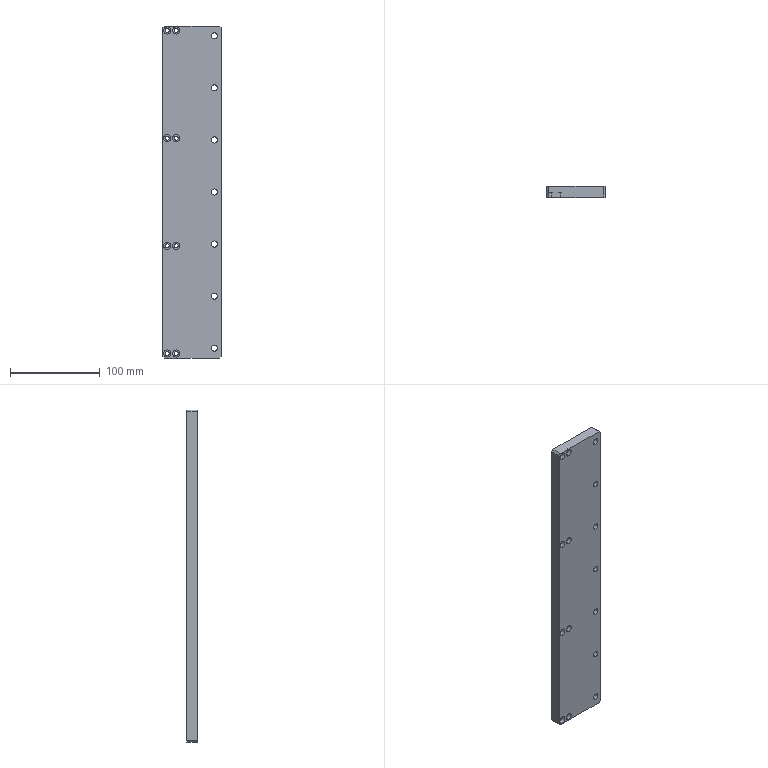Part | SolidWorks | features HoleWzd 2, Chamfer 1, Extrusion 1, LPattern 1 | 1 solid | 64 faces | box 65 x 12 x 370 mm | volume 282662 mm3 | cylinder 46 | plane 18 | commonest cylinder face diameters 4.5 x16 8 x16 6.8 x14